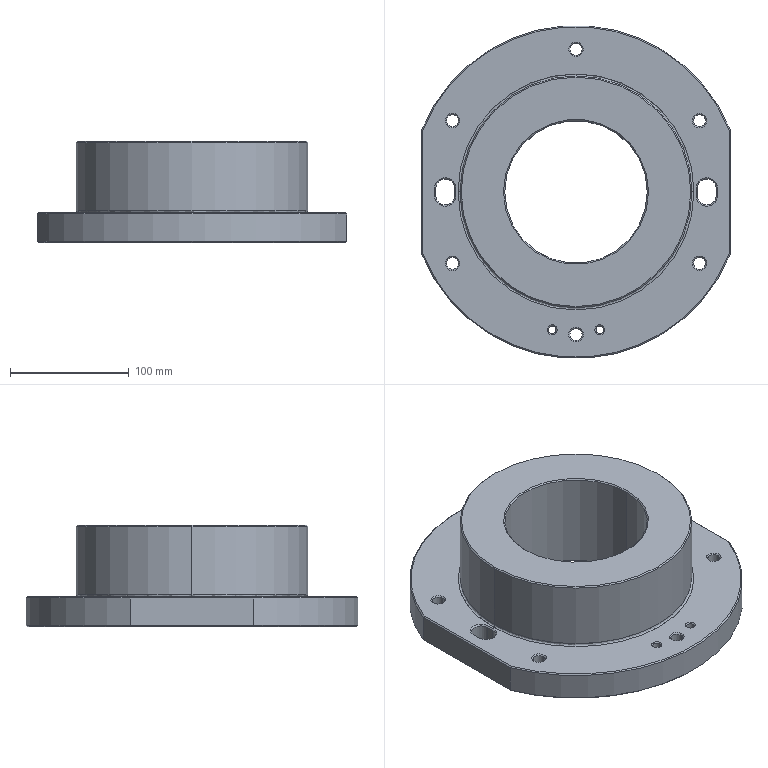Part | SolidWorks | features BaseBody 1 | 1 solid | 140 faces | box 260 x 280 x 85 mm | volume 2297762 mm3 | cone 67 | cylinder 42 | plane 29 | spline 2 | commonest cylinder face diameters 6.5 x20 10.2 x12 16 x4 120 x2 195 x2 280 x2